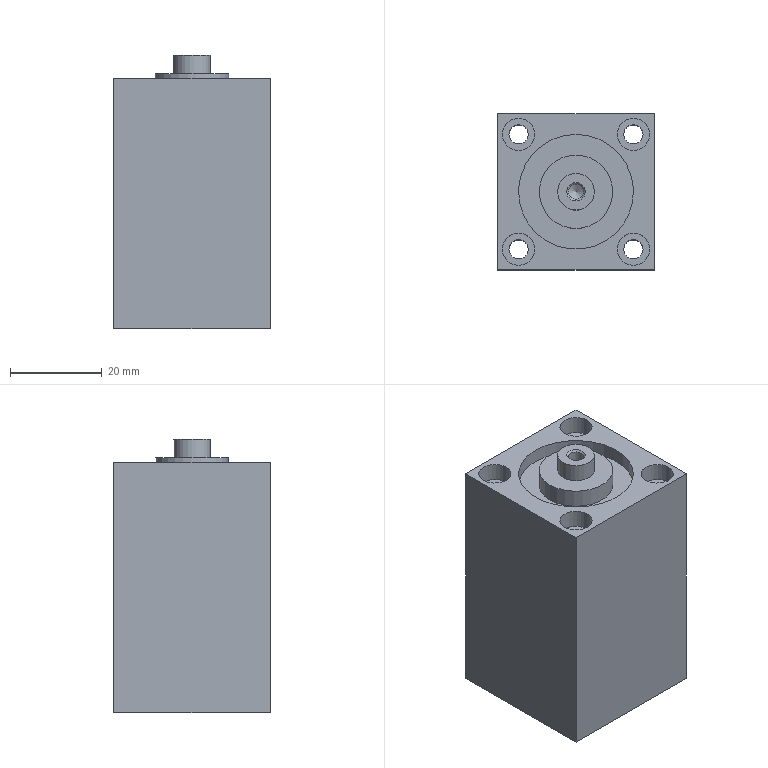Part | NX | features DATUM_CSYS 8, EXTRUDE 7, SKETCH 7, HOLE PACKAGE 1, Instance Feature 1, Mirror Feature 1, SIMPLE HOLE 1, SUBTRACT 1, SYMBOLIC_THREAD 1 | 2 solids | 38 faces | box 34 x 34 x 59.5 mm | volume 58620 mm3 | plane 19 | cylinder 17 | cone 2 | commonest cylinder face diameters 7 x8 4.2 x4 8 x2 3.3 x1 16 x1 25 x1
STEP:
#1=CARTESIAN_POINT('',(4.,0.,59.5));
#2=VERTEX_POINT('',#1);
#3=CARTESIAN_POINT('',(0.,0.,59.5));
#4=DIRECTION('',(0.,0.,1.));
#5=DIRECTION('',(1.,0.,0.));
#6=AXIS2_PLACEMENT_3D('',#3,#4,#5);
#7=CIRCLE('',#6,4.);
#8=EDGE_CURVE('',#2,#2,#7,.T.);
#9=ORIENTED_EDGE('',*,*,#8,.F.);
#10=EDGE_LOOP('',(#9));
#11=FACE_BOUND('',#10,.T.);
#12=CARTESIAN_POINT('',(4.,0.,5.5));
#13=VERTEX_POINT('',#12);
#14=CARTESIAN_POINT('',(0.,0.,5.5));
#15=DIRECTION('',(0.,0.,1.));
#16=DIRECTION('',(1.,0.,0.));
#17=AXIS2_PLACEMENT_3D('',#14,#15,#16);
#18=CIRCLE('',#17,4.);
#19=EDGE_CURVE('',#13,#13,#18,.T.);
#20=ORIENTED_EDGE('',*,*,#19,.T.);
#21=EDGE_LOOP('',(#20));
#22=FACE_BOUND('',#21,.T.);
#23=CARTESIAN_POINT('',(0.,0.,59.5));
#24=DIRECTION('',(0.,0.,-1.));
#25=DIRECTION('',(-1.,0.,0.));
#26=AXIS2_PLACEMENT_3D('',#23,#24,#25);
#27=CYLINDRICAL_SURFACE('',#26,4.);
#28=ADVANCED_FACE('',(#11,#22),#27,.T.);
#29=CARTESIAN_POINT('',(2.,0.,59.5));
#30=VERTEX_POINT('',#29);
#31=CARTESIAN_POINT('',(0.,0.,59.5));
#32=DIRECTION('',(0.,0.,1.));
#33=DIRECTION('',(1.,0.,0.));
#34=AXIS2_PLACEMENT_3D('',#31,#32,#33);
#35=CIRCLE('',#34,2.);
#36=EDGE_CURVE('',#30,#30,#35,.F.);
#37=ORIENTED_EDGE('',*,*,#36,.T.);
#38=EDGE_LOOP('',(#37));
#39=FACE_BOUND('',#38,.T.);
#40=ORIENTED_EDGE('',*,*,#8,.T.);
#41=EDGE_LOOP('',(#40));
#42=FACE_BOUND('',#41,.T.);
#43=CARTESIAN_POINT('',(0.,0.,59.5));
#44=DIRECTION('',(0.,0.,1.));
#45=DIRECTION('',(1.,0.,0.));
#46=AXIS2_PLACEMENT_3D('',#43,#44,#45);
#47=PLANE('',#46);
#48=ADVANCED_FACE('',(#39,#42),#47,.T.);
#49=ORIENTED_EDGE('',*,*,#19,.F.);
#50=EDGE_LOOP('',(#49));
#51=FACE_BOUND('',#50,.T.);
#52=CARTESIAN_POINT('',(0.,0.,5.5));
#53=DIRECTION('',(0.,0.,1.));
#54=DIRECTION('',(1.,0.,0.));
#55=AXIS2_PLACEMENT_3D('',#52,#53,#54);
#56=PLANE('',#55);
#57=ADVANCED_FACE('',(#51),#56,.F.);
#58=CARTESIAN_POINT('',(-1.65,0.,47.5));
#59=VERTEX_POINT('',#58);
#60=CARTESIAN_POINT('',(0.,0.,47.5));
#61=DIRECTION('',(0.,0.,-1.));
#62=DIRECTION('',(-1.,0.,0.));
#63=AXIS2_PLACEMENT_3D('',#60,#61,#62);
#64=CIRCLE('',#63,1.65);
#65=EDGE_CURVE('',#59,#59,#64,.F.);
#66=ORIENTED_EDGE('',*,*,#65,.T.);
#67=EDGE_LOOP('',(#66));
#68=FACE_BOUND('',#67,.T.);
#69=CARTESIAN_POINT('',(0.,0.,46.509));
#70=VERTEX_POINT('',#69);
#71=VERTEX_LOOP('',#70);
#72=FACE_BOUND('',#71,.T.);
#73=CARTESIAN_POINT('',(0.,0.,47.5));
#74=DIRECTION('',(0.,0.,1.));
#75=DIRECTION('',(1.,0.,0.));
#76=AXIS2_PLACEMENT_3D('',#73,#74,#75);
#77=CONICAL_SURFACE('',#76,1.65,1.03);
#78=ADVANCED_FACE('',(#68,#72),#77,.F.);
#79=CARTESIAN_POINT('',(1.65,0.,59.15));
#80=VERTEX_POINT('',#79);
#81=CARTESIAN_POINT('',(0.,0.,59.15));
#82=DIRECTION('',(0.,0.,1.));
#83=DIRECTION('',(1.,0.,0.));
#84=AXIS2_PLACEMENT_3D('',#81,#82,#83);
#85=CIRCLE('',#84,1.65);
#86=EDGE_CURVE('',#80,#80,#85,.T.);
#87=ORIENTED_EDGE('',*,*,#86,.T.);
#88=EDGE_LOOP('',(#87));
#89=FACE_BOUND('',#88,.T.);
#90=ORIENTED_EDGE('',*,*,#65,.F.);
#91=EDGE_LOOP('',(#90));
#92=FACE_BOUND('',#91,.T.);
#93=CARTESIAN_POINT('',(0.,0.,59.5));
#94=DIRECTION('',(0.,0.,-1.));
#95=DIRECTION('',(-1.,0.,0.));
#96=AXIS2_PLACEMENT_3D('',#93,#94,#95);
#97=CYLINDRICAL_SURFACE('',#96,1.65);
#98=ADVANCED_FACE('',(#89,#92),#97,.F.);
#99=ORIENTED_EDGE('',*,*,#86,.F.);
#100=EDGE_LOOP('',(#99));
#101=FACE_BOUND('',#100,.T.);
#102=ORIENTED_EDGE('',*,*,#36,.F.);
#103=EDGE_LOOP('',(#102));
#104=FACE_BOUND('',#103,.T.);
#105=CARTESIAN_POINT('',(0.,0.,59.5));
#106=DIRECTION('',(0.,0.,1.));
#107=DIRECTION('',(1.,0.,0.));
#108=AXIS2_PLACEMENT_3D('',#105,#106,#107);
#109=CONICAL_SURFACE('',#108,2.,0.7854);
#110=ADVANCED_FACE('',(#101,#104),#109,.F.);
#111=CLOSED_SHELL('',(#28,#48,#57,#78,#98,#110));
#112=MANIFOLD_SOLID_BREP('',#111);
#113=CARTESIAN_POINT('',(-16.,12.5,54.5));
#114=VERTEX_POINT('',#113);
#115=CARTESIAN_POINT('',(-12.5,12.5,54.5));
#116=DIRECTION('',(0.,0.,-1.));
#117=DIRECTION('',(-1.,0.,0.));
#118=AXIS2_PLACEMENT_3D('',#115,#116,#117);
#119=CIRCLE('',#118,3.5);
#120=EDGE_CURVE('',#114,#114,#119,.T.);
#121=ORIENTED_EDGE('',*,*,#120,.T.);
#122=EDGE_LOOP('',(#121));
#123=FACE_BOUND('',#122,.T.);
#124=CARTESIAN_POINT('',(16.,12.5,54.5));
#125=VERTEX_POINT('',#124);
#126=CARTESIAN_POINT('',(12.5,12.5,54.5));
#127=DIRECTION('',(0.,0.,1.));
#128=DIRECTION('',(1.,0.,0.));
#129=AXIS2_PLACEMENT_3D('',#126,#127,#128);
#130=CIRCLE('',#129,3.5);
#131=EDGE_CURVE('',#125,#125,#130,.T.);
#132=ORIENTED_EDGE('',*,*,#131,.F.);
#133=EDGE_LOOP('',(#132));
#134=FACE_BOUND('',#133,.T.);
#135=CARTESIAN_POINT('',(0.,12.5,54.5));
#136=VERTEX_POINT('',#135);
#137=CARTESIAN_POINT('',(0.,0.,54.5));
#138=DIRECTION('',(0.,0.,1.));
#139=DIRECTION('',(0.,1.,0.));
#140=AXIS2_PLACEMENT_3D('',#137,#138,#139);
#141=CIRCLE('',#140,12.5);
#142=EDGE_CURVE('',#136,#136,#141,.T.);
#143=ORIENTED_EDGE('',*,*,#142,.F.);
#144=EDGE_LOOP('',(#143));
#145=FACE_BOUND('',#144,.T.);
#146=CARTESIAN_POINT('',(-17.,17.,54.5));
#147=VERTEX_POINT('',#146);
#148=CARTESIAN_POINT('',(-17.,-17.,54.5));
#149=VERTEX_POINT('',#148);
#150=CARTESIAN_POINT('',(-17.,17.,54.5));
#151=DIRECTION('',(0.,-1.,0.));
#152=VECTOR('',#151,1000.);
#153=LINE('',#150,#152);
#154=EDGE_CURVE('',#147,#149,#153,.T.);
#155=ORIENTED_EDGE('',*,*,#154,.T.);
#156=CARTESIAN_POINT('',(17.,-17.,54.5));
#157=VERTEX_POINT('',#156);
#158=CARTESIAN_POINT('',(-17.,-17.,54.5));
#159=DIRECTION('',(1.,0.,0.));
#160=VECTOR('',#159,1000.);
#161=LINE('',#158,#160);
#162=EDGE_CURVE('',#149,#157,#161,.T.);
#163=ORIENTED_EDGE('',*,*,#162,.T.);
#164=CARTESIAN_POINT('',(17.,17.,54.5));
#165=VERTEX_POINT('',#164);
#166=CARTESIAN_POINT('',(17.,-17.,54.5));
#167=DIRECTION('',(0.,1.,0.));
#168=VECTOR('',#167,1000.);
#169=LINE('',#166,#168);
#170=EDGE_CURVE('',#157,#165,#169,.T.);
#171=ORIENTED_EDGE('',*,*,#170,.T.);
#172=CARTESIAN_POINT('',(17.,17.,54.5));
#173=DIRECTION('',(-1.,0.,0.));
#174=VECTOR('',#173,1000.);
#175=LINE('',#172,#174);
#176=EDGE_CURVE('',#165,#147,#175,.T.);
#177=ORIENTED_EDGE('',*,*,#176,.T.);
#178=EDGE_LOOP('',(#155,#163,#171,#177));
#179=FACE_BOUND('',#178,.T.);
#180=CARTESIAN_POINT('',(-16.,-12.5,54.5));
#181=VERTEX_POINT('',#180);
#182=CARTESIAN_POINT('',(-12.5,-12.5,54.5));
#183=DIRECTION('',(0.,0.,1.));
#184=DIRECTION('',(-1.,0.,0.));
#185=AXIS2_PLACEMENT_3D('',#182,#183,#184);
#186=CIRCLE('',#185,3.5);
#187=EDGE_CURVE('',#181,#181,#186,.T.);
#188=ORIENTED_EDGE('',*,*,#187,.F.);
#189=EDGE_LOOP('',(#188));
#190=FACE_BOUND('',#189,.T.);
#191=CARTESIAN_POINT('',(16.,-12.5,54.5));
#192=VERTEX_POINT('',#191);
#193=CARTESIAN_POINT('',(12.5,-12.5,54.5));
#194=DIRECTION('',(0.,0.,-1.));
#195=DIRECTION('',(1.,0.,0.));
#196=AXIS2_PLACEMENT_3D('',#193,#194,#195);
#197=CIRCLE('',#196,3.5);
#198=EDGE_CURVE('',#192,#192,#197,.T.);
#199=ORIENTED_EDGE('',*,*,#198,.T.);
#200=EDGE_LOOP('',(#199));
#201=FACE_BOUND('',#200,.T.);
#202=CARTESIAN_POINT('',(0.,0.,54.5));
#203=DIRECTION('',(0.,0.,1.));
#204=DIRECTION('',(1.,0.,0.));
#205=AXIS2_PLACEMENT_3D('',#202,#203,#204);
#206=PLANE('',#205);
#207=ADVANCED_FACE('',(#123,#134,#145,#179,#190,#201),#206,.T.);
#208=CARTESIAN_POINT('',(-16.,12.5,0.));
#209=VERTEX_POINT('',#208);
#210=CARTESIAN_POINT('',(-12.5,12.5,0.));
#211=DIRECTION('',(0.,0.,-1.));
#212=DIRECTION('',(-1.,0.,0.));
#213=AXIS2_PLACEMENT_3D('',#210,#211,#212);
#214=CIRCLE('',#213,3.5);
#215=EDGE_CURVE('',#209,#209,#214,.T.);
#216=ORIENTED_EDGE('',*,*,#215,.F.);
#217=EDGE_LOOP('',(#216));
#218=FACE_BOUND('',#217,.T.);
#219=CARTESIAN_POINT('',(16.,12.5,0.));
#220=VERTEX_POINT('',#219);
#221=CARTESIAN_POINT('',(12.5,12.5,0.));
#222=DIRECTION('',(0.,0.,1.));
#223=DIRECTION('',(1.,0.,0.));
#224=AXIS2_PLACEMENT_3D('',#221,#222,#223);
#225=CIRCLE('',#224,3.5);
#226=EDGE_CURVE('',#220,#220,#225,.T.);
#227=ORIENTED_EDGE('',*,*,#226,.T.);
#228=EDGE_LOOP('',(#227));
#229=FACE_BOUND('',#228,.T.);
#230=CARTESIAN_POINT('',(-17.,17.,0.));
#231=VERTEX_POINT('',#230);
#232=CARTESIAN_POINT('',(-17.,-17.,0.));
#233=VERTEX_POINT('',#232);
#234=CARTESIAN_POINT('',(-17.,17.,0.));
#235=DIRECTION('',(0.,-1.,0.));
#236=VECTOR('',#235,1000.);
#237=LINE('',#234,#236);
#238=EDGE_CURVE('',#231,#233,#237,.T.);
#239=ORIENTED_EDGE('',*,*,#238,.F.);
#240=CARTESIAN_POINT('',(17.,17.,0.));
#241=VERTEX_POINT('',#240);
#242=CARTESIAN_POINT('',(17.,17.,0.));
#243=DIRECTION('',(-1.,0.,0.));
#244=VECTOR('',#243,1000.);
#245=LINE('',#242,#244);
#246=EDGE_CURVE('',#241,#231,#245,.T.);
#247=ORIENTED_EDGE('',*,*,#246,.F.);
#248=CARTESIAN_POINT('',(17.,-17.,0.));
#249=VERTEX_POINT('',#248);
#250=CARTESIAN_POINT('',(17.,-17.,0.));
#251=DIRECTION('',(0.,1.,0.));
#252=VECTOR('',#251,1000.);
#253=LINE('',#250,#252);
#254=EDGE_CURVE('',#249,#241,#253,.T.);
#255=ORIENTED_EDGE('',*,*,#254,.F.);
#256=CARTESIAN_POINT('',(-17.,-17.,0.));
#257=DIRECTION('',(1.,0.,0.));
#258=VECTOR('',#257,1000.);
#259=LINE('',#256,#258);
#260=EDGE_CURVE('',#233,#249,#259,.T.);
#261=ORIENTED_EDGE('',*,*,#260,.F.);
#262=EDGE_LOOP('',(#239,#247,#255,#261));
#263=FACE_BOUND('',#262,.T.);
#264=CARTESIAN_POINT('',(-16.,-12.5,0.));
#265=VERTEX_POINT('',#264);
#266=CARTESIAN_POINT('',(-12.5,-12.5,0.));
#267=DIRECTION('',(0.,0.,1.));
#268=DIRECTION('',(-1.,0.,0.));
#269=AXIS2_PLACEMENT_3D('',#266,#267,#268);
#270=CIRCLE('',#269,3.5);
#271=EDGE_CURVE('',#265,#265,#270,.T.);
#272=ORIENTED_EDGE('',*,*,#271,.T.);
#273=EDGE_LOOP('',(#272));
#274=FACE_BOUND('',#273,.T.);
#275=CARTESIAN_POINT('',(16.,-12.5,0.));
#276=VERTEX_POINT('',#275);
#277=CARTESIAN_POINT('',(12.5,-12.5,0.));
#278=DIRECTION('',(0.,0.,-1.));
#279=DIRECTION('',(1.,0.,0.));
#280=AXIS2_PLACEMENT_3D('',#277,#278,#279);
#281=CIRCLE('',#280,3.5);
#282=EDGE_CURVE('',#276,#276,#281,.T.);
#283=ORIENTED_EDGE('',*,*,#282,.F.);
#284=EDGE_LOOP('',(#283));
#285=FACE_BOUND('',#284,.T.);
#286=CARTESIAN_POINT('',(0.,0.,0.));
#287=DIRECTION('',(0.,0.,1.));
#288=DIRECTION('',(1.,0.,0.));
#289=AXIS2_PLACEMENT_3D('',#286,#287,#288);
#290=PLANE('',#289);
#291=ADVANCED_FACE('',(#218,#229,#263,#274,#285),#290,.F.);
#292=ORIENTED_EDGE('',*,*,#238,.T.);
#293=CARTESIAN_POINT('',(-17.,-17.,54.5));
#294=DIRECTION('',(0.,0.,-1.));
#295=VECTOR('',#294,1000.);
#296=LINE('',#293,#295);
#297=EDGE_CURVE('',#149,#233,#296,.T.);
#298=ORIENTED_EDGE('',*,*,#297,.F.);
#299=ORIENTED_EDGE('',*,*,#154,.F.);
#300=CARTESIAN_POINT('',(-17.,17.,54.5));
#301=DIRECTION('',(0.,0.,-1.));
#302=VECTOR('',#301,1000.);
#303=LINE('',#300,#302);
#304=EDGE_CURVE('',#147,#231,#303,.T.);
#305=ORIENTED_EDGE('',*,*,#304,.T.);
#306=EDGE_LOOP('',(#292,#298,#299,#305));
#307=FACE_BOUND('',#306,.T.);
#308=CARTESIAN_POINT('',(-17.,17.,54.5));
#309=DIRECTION('',(1.,0.,0.));
#310=DIRECTION('',(0.,0.,-1.));
#311=AXIS2_PLACEMENT_3D('',#308,#309,#310);
#312=PLANE('',#311);
#313=ADVANCED_FACE('',(#307),#312,.F.);
#314=ORIENTED_EDGE('',*,*,#260,.T.);
#315=CARTESIAN_POINT('',(17.,-17.,54.5));
#316=DIRECTION('',(0.,0.,-1.));
#317=VECTOR('',#316,1000.);
#318=LINE('',#315,#317);
#319=EDGE_CURVE('',#157,#249,#318,.T.);
#320=ORIENTED_EDGE('',*,*,#319,.F.);
#321=ORIENTED_EDGE('',*,*,#162,.F.);
#322=ORIENTED_EDGE('',*,*,#297,.T.);
#323=EDGE_LOOP('',(#314,#320,#321,#322));
#324=FACE_BOUND('',#323,.T.);
#325=CARTESIAN_POINT('',(-17.,-17.,54.5));
#326=DIRECTION('',(0.,1.,0.));
#327=DIRECTION('',(0.,0.,1.));
#328=AXIS2_PLACEMENT_3D('',#325,#326,#327);
#329=PLANE('',#328);
#330=ADVANCED_FACE('',(#324),#329,.F.);
#331=ORIENTED_EDGE('',*,*,#254,.T.);
#332=CARTESIAN_POINT('',(17.,17.,54.5));
#333=DIRECTION('',(0.,0.,-1.));
#334=VECTOR('',#333,1000.);
#335=LINE('',#332,#334);
#336=EDGE_CURVE('',#165,#241,#335,.T.);
#337=ORIENTED_EDGE('',*,*,#336,.F.);
#338=ORIENTED_EDGE('',*,*,#170,.F.);
#339=ORIENTED_EDGE('',*,*,#319,.T.);
#340=EDGE_LOOP('',(#331,#337,#338,#339));
#341=FACE_BOUND('',#340,.T.);
#342=CARTESIAN_POINT('',(17.,-17.,54.5));
#343=DIRECTION('',(-1.,0.,0.));
#344=DIRECTION('',(0.,0.,1.));
#345=AXIS2_PLACEMENT_3D('',#342,#343,#344);
#346=PLANE('',#345);
#347=ADVANCED_FACE('',(#341),#346,.F.);
#348=ORIENTED_EDGE('',*,*,#246,.T.);
#349=ORIENTED_EDGE('',*,*,#304,.F.);
#350=ORIENTED_EDGE('',*,*,#176,.F.);
#351=ORIENTED_EDGE('',*,*,#336,.T.);
#352=EDGE_LOOP('',(#348,#349,#350,#351));
#353=FACE_BOUND('',#352,.T.);
#354=CARTESIAN_POINT('',(17.,17.,54.5));
#355=DIRECTION('',(0.,-1.,0.));
#356=DIRECTION('',(0.,0.,-1.));
#357=AXIS2_PLACEMENT_3D('',#354,#355,#356);
#358=PLANE('',#357);
#359=ADVANCED_FACE('',(#353),#358,.F.);
#360=CARTESIAN_POINT('',(0.,12.5,51.5));
#361=VERTEX_POINT('',#360);
#362=CARTESIAN_POINT('',(0.,0.,51.5));
#363=DIRECTION('',(0.,0.,1.));
#364=DIRECTION('',(0.,1.,0.));
#365=AXIS2_PLACEMENT_3D('',#362,#363,#364);
#366=CIRCLE('',#365,12.5);
#367=EDGE_CURVE('',#361,#361,#366,.F.);
#368=ORIENTED_EDGE('',*,*,#367,.T.);
#369=EDGE_LOOP('',(#368));
#370=FACE_BOUND('',#369,.T.);
#371=ORIENTED_EDGE('',*,*,#142,.T.);
#372=EDGE_LOOP('',(#371));
#373=FACE_BOUND('',#372,.T.);
#374=CARTESIAN_POINT('',(0.,0.,51.5));
#375=DIRECTION('',(0.,0.,1.));
#376=DIRECTION('',(1.,0.,0.));
#377=AXIS2_PLACEMENT_3D('',#374,#375,#376);
#378=CYLINDRICAL_SURFACE('',#377,12.5);
#379=ADVANCED_FACE('',(#370,#373),#378,.F.);
#380=CARTESIAN_POINT('',(8.,0.,51.5));
#381=VERTEX_POINT('',#380);
#382=CARTESIAN_POINT('',(0.,0.,51.5));
#383=DIRECTION('',(0.,0.,1.));
#384=DIRECTION('',(1.,0.,0.));
#385=AXIS2_PLACEMENT_3D('',#382,#383,#384);
#386=CIRCLE('',#385,8.);
#387=EDGE_CURVE('',#381,#381,#386,.T.);
#388=ORIENTED_EDGE('',*,*,#387,.F.);
#389=EDGE_LOOP('',(#388));
#390=FACE_BOUND('',#389,.T.);
#391=ORIENTED_EDGE('',*,*,#367,.F.);
#392=EDGE_LOOP('',(#391));
#393=FACE_BOUND('',#392,.T.);
#394=CARTESIAN_POINT('',(0.,0.,51.5));
#395=DIRECTION('',(0.,0.,1.));
#396=DIRECTION('',(1.,0.,0.));
#397=AXIS2_PLACEMENT_3D('',#394,#395,#396);
#398=PLANE('',#397);
#399=ADVANCED_FACE('',(#390,#393),#398,.T.);
#400=CARTESIAN_POINT('',(8.,0.,55.5));
#401=VERTEX_POINT('',#400);
#402=CARTESIAN_POINT('',(0.,0.,55.5));
#403=DIRECTION('',(0.,0.,1.));
#404=DIRECTION('',(1.,0.,0.));
#405=AXIS2_PLACEMENT_3D('',#402,#403,#404);
#406=CIRCLE('',#405,8.);
#407=EDGE_CURVE('',#401,#401,#406,.T.);
#408=ORIENTED_EDGE('',*,*,#407,.F.);
#409=EDGE_LOOP('',(#408));
#410=FACE_BOUND('',#409,.T.);
#411=ORIENTED_EDGE('',*,*,#387,.T.);
#412=EDGE_LOOP('',(#411));
#413=FACE_BOUND('',#412,.T.);
#414=CARTESIAN_POINT('',(0.,0.,55.5));
#415=DIRECTION('',(0.,0.,-1.));
#416=DIRECTION('',(-1.,0.,0.));
#417=AXIS2_PLACEMENT_3D('',#414,#415,#416);
#418=CYLINDRICAL_SURFACE('',#417,8.);
#419=ADVANCED_FACE('',(#410,#413),#418,.T.);
#420=CARTESIAN_POINT('',(4.,0.,55.5));
#421=VERTEX_POINT('',#420);
#422=CARTESIAN_POINT('',(0.,0.,55.5));
#423=DIRECTION('',(0.,0.,1.));
#424=DIRECTION('',(1.,0.,0.));
#425=AXIS2_PLACEMENT_3D('',#422,#423,#424);
#426=CIRCLE('',#425,4.);
#427=EDGE_CURVE('',#421,#421,#426,.F.);
#428=ORIENTED_EDGE('',*,*,#427,.T.);
#429=EDGE_LOOP('',(#428));
#430=FACE_BOUND('',#429,.T.);
#431=ORIENTED_EDGE('',*,*,#407,.T.);
#432=EDGE_LOOP('',(#431));
#433=FACE_BOUND('',#432,.T.);
#434=CARTESIAN_POINT('',(0.,0.,55.5));
#435=DIRECTION('',(0.,0.,1.));
#436=DIRECTION('',(1.,0.,0.));
#437=AXIS2_PLACEMENT_3D('',#434,#435,#436);
#438=PLANE('',#437);
#439=ADVANCED_FACE('',(#430,#433),#438,.T.);
#440=CARTESIAN_POINT('',(16.,12.5,4.));
#441=VERTEX_POINT('',#440);
#442=CARTESIAN_POINT('',(12.5,12.5,4.));
#443=DIRECTION('',(0.,0.,1.));
#444=DIRECTION('',(1.,0.,0.));
#445=AXIS2_PLACEMENT_3D('',#442,#443,#444);
#446=CIRCLE('',#445,3.5);
#447=EDGE_CURVE('',#441,#441,#446,.F.);
#448=ORIENTED_EDGE('',*,*,#447,.F.);
#449=EDGE_LOOP('',(#448));
#450=FACE_BOUND('',#449,.T.);
#451=ORIENTED_EDGE('',*,*,#226,.F.);
#452=EDGE_LOOP('',(#451));
#453=FACE_BOUND('',#452,.T.);
#454=CARTESIAN_POINT('',(12.5,12.5,4.));
#455=DIRECTION('',(0.,0.,-1.));
#456=DIRECTION('',(-1.,0.,0.));
#457=AXIS2_PLACEMENT_3D('',#454,#455,#456);
#458=CYLINDRICAL_SURFACE('',#457,3.5);
#459=ADVANCED_FACE('',(#450,#453),#458,.F.);
#460=CARTESIAN_POINT('',(14.6,12.5,4.));
#461=VERTEX_POINT('',#460);
#462=CARTESIAN_POINT('',(12.5,12.5,4.));
#463=DIRECTION('',(0.,0.,1.));
#464=DIRECTION('',(1.,0.,0.));
#465=AXIS2_PLACEMENT_3D('',#462,#463,#464);
#466=CIRCLE('',#465,2.1);
#467=EDGE_CURVE('',#461,#461,#466,.T.);
#468=ORIENTED_EDGE('',*,*,#467,.T.);
#469=EDGE_LOOP('',(#468));
#470=FACE_BOUND('',#469,.T.);
#471=ORIENTED_EDGE('',*,*,#447,.T.);
#472=EDGE_LOOP('',(#471));
#473=FACE_BOUND('',#472,.T.);
#474=CARTESIAN_POINT('',(12.5,12.5,4.));
#475=DIRECTION('',(0.,0.,1.));
#476=DIRECTION('',(1.,0.,0.));
#477=AXIS2_PLACEMENT_3D('',#474,#475,#476);
#478=PLANE('',#477);
#479=ADVANCED_FACE('',(#470,#473),#478,.F.);
#480=CARTESIAN_POINT('',(-16.,12.5,4.));
#481=VERTEX_POINT('',#480);
#482=CARTESIAN_POINT('',(-12.5,12.5,4.));
#483=DIRECTION('',(0.,0.,-1.));
#484=DIRECTION('',(-1.,0.,0.));
#485=AXIS2_PLACEMENT_3D('',#482,#483,#484);
#486=CIRCLE('',#485,3.5);
#487=EDGE_CURVE('',#481,#481,#486,.F.);
#488=ORIENTED_EDGE('',*,*,#487,.T.);
#489=EDGE_LOOP('',(#488));
#490=FACE_BOUND('',#489,.T.);
#491=ORIENTED_EDGE('',*,*,#215,.T.);
#492=EDGE_LOOP('',(#491));
#493=FACE_BOUND('',#492,.T.);
#494=CARTESIAN_POINT('',(-12.5,12.5,4.));
#495=DIRECTION('',(0.,0.,-1.));
#496=DIRECTION('',(-1.,0.,0.));
#497=AXIS2_PLACEMENT_3D('',#494,#495,#496);
#498=CYLINDRICAL_SURFACE('',#497,3.5);
#499=ADVANCED_FACE('',(#490,#493),#498,.F.);
#500=CARTESIAN_POINT('',(-14.6,12.5,4.));
#501=VERTEX_POINT('',#500);
#502=CARTESIAN_POINT('',(-12.5,12.5,4.));
#503=DIRECTION('',(0.,0.,-1.));
#504=DIRECTION('',(-1.,0.,0.));
#505=AXIS2_PLACEMENT_3D('',#502,#503,#504);
#506=CIRCLE('',#505,2.1);
#507=EDGE_CURVE('',#501,#501,#506,.T.);
#508=ORIENTED_EDGE('',*,*,#507,.F.);
#509=EDGE_LOOP('',(#508));
#510=FACE_BOUND('',#509,.T.);
#511=ORIENTED_EDGE('',*,*,#487,.F.);
#512=EDGE_LOOP('',(#511));
#513=FACE_BOUND('',#512,.T.);
#514=CARTESIAN_POINT('',(-12.5,12.5,4.));
#515=DIRECTION('',(0.,0.,-1.));
#516=DIRECTION('',(-1.,0.,0.));
#517=AXIS2_PLACEMENT_3D('',#514,#515,#516);
#518=PLANE('',#517);
#519=ADVANCED_FACE('',(#510,#513),#518,.T.);
#520=CARTESIAN_POINT('',(-16.,-12.5,4.));
#521=VERTEX_POINT('',#520);
#522=CARTESIAN_POINT('',(-12.5,-12.5,4.));
#523=DIRECTION('',(0.,0.,1.));
#524=DIRECTION('',(-1.,0.,0.));
#525=AXIS2_PLACEMENT_3D('',#522,#523,#524);
#526=CIRCLE('',#525,3.5);
#527=EDGE_CURVE('',#521,#521,#526,.F.);
#528=ORIENTED_EDGE('',*,*,#527,.F.);
#529=EDGE_LOOP('',(#528));
#530=FACE_BOUND('',#529,.T.);
#531=ORIENTED_EDGE('',*,*,#271,.F.);
#532=EDGE_LOOP('',(#531));
#533=FACE_BOUND('',#532,.T.);
#534=CARTESIAN_POINT('',(-12.5,-12.5,4.));
#535=DIRECTION('',(0.,0.,-1.));
#536=DIRECTION('',(-1.,0.,0.));
#537=AXIS2_PLACEMENT_3D('',#534,#535,#536);
#538=CYLINDRICAL_SURFACE('',#537,3.5);
#539=ADVANCED_FACE('',(#530,#533),#538,.F.);
#540=CARTESIAN_POINT('',(-10.4,-12.5,4.));
#541=VERTEX_POINT('',#540);
#542=CARTESIAN_POINT('',(-12.5,-12.5,4.));
#543=DIRECTION('',(0.,0.,1.));
#544=DIRECTION('',(1.,0.,0.));
#545=AXIS2_PLACEMENT_3D('',#542,#543,#544);
#546=CIRCLE('',#545,2.1);
#547=EDGE_CURVE('',#541,#541,#546,.T.);
#548=ORIENTED_EDGE('',*,*,#547,.T.);
#549=EDGE_LOOP('',(#548));
#550=FACE_BOUND('',#549,.T.);
#551=ORIENTED_EDGE('',*,*,#527,.T.);
#552=EDGE_LOOP('',(#551));
#553=FACE_BOUND('',#552,.T.);
#554=CARTESIAN_POINT('',(-12.5,-12.5,4.));
#555=DIRECTION('',(0.,0.,1.));
#556=DIRECTION('',(1.,0.,0.));
#557=AXIS2_PLACEMENT_3D('',#554,#555,#556);
#558=PLANE('',#557);
#559=ADVANCED_FACE('',(#550,#553),#558,.F.);
#560=CARTESIAN_POINT('',(16.,-12.5,4.));
#561=VERTEX_POINT('',#560);
#562=CARTESIAN_POINT('',(12.5,-12.5,4.));
#563=DIRECTION('',(0.,0.,-1.));
#564=DIRECTION('',(1.,0.,0.));
#565=AXIS2_PLACEMENT_3D('',#562,#563,#564);
#566=CIRCLE('',#565,3.5);
#567=EDGE_CURVE('',#561,#561,#566,.F.);
#568=ORIENTED_EDGE('',*,*,#567,.T.);
#569=EDGE_LOOP('',(#568));
#570=FACE_BOUND('',#569,.T.);
#571=ORIENTED_EDGE('',*,*,#282,.T.);
#572=EDGE_LOOP('',(#571));
#573=FACE_BOUND('',#572,.T.);
#574=CARTESIAN_POINT('',(12.5,-12.5,4.));
#575=DIRECTION('',(0.,0.,-1.));
#576=DIRECTION('',(-1.,0.,0.));
#577=AXIS2_PLACEMENT_3D('',#574,#575,#576);
#578=CYLINDRICAL_SURFACE('',#577,3.5);
#579=ADVANCED_FACE('',(#570,#573),#578,.F.);
#580=CARTESIAN_POINT('',(10.4,-12.5,4.));
#581=VERTEX_POINT('',#580);
#582=CARTESIAN_POINT('',(12.5,-12.5,4.));
#583=DIRECTION('',(0.,0.,-1.));
#584=DIRECTION('',(-1.,0.,0.));
#585=AXIS2_PLACEMENT_3D('',#582,#583,#584);
#586=CIRCLE('',#585,2.1);
#587=EDGE_CURVE('',#581,#581,#586,.T.);
#588=ORIENTED_EDGE('',*,*,#587,.F.);
#589=EDGE_LOOP('',(#588));
#590=FACE_BOUND('',#589,.T.);
#591=ORIENTED_EDGE('',*,*,#567,.F.);
#592=EDGE_LOOP('',(#591));
#593=FACE_BOUND('',#592,.T.);
#594=CARTESIAN_POINT('',(12.5,-12.5,4.));
#595=DIRECTION('',(0.,0.,-1.));
#596=DIRECTION('',(-1.,0.,0.));
#597=AXIS2_PLACEMENT_3D('',#594,#595,#596);
#598=PLANE('',#597);
#599=ADVANCED_FACE('',(#590,#593),#598,.T.);
#600=CARTESIAN_POINT('',(16.,12.5,50.5));
#601=VERTEX_POINT('',#600);
#602=CARTESIAN_POINT('',(12.5,12.5,50.5));
#603=DIRECTION('',(0.,0.,1.));
#604=DIRECTION('',(1.,0.,0.));
#605=AXIS2_PLACEMENT_3D('',#602,#603,#604);
#606=CIRCLE('',#605,3.5);
#607=EDGE_CURVE('',#601,#601,#606,.F.);
#608=ORIENTED_EDGE('',*,*,#607,.T.);
#609=EDGE_LOOP('',(#608));
#610=FACE_BOUND('',#609,.T.);
#611=ORIENTED_EDGE('',*,*,#131,.T.);
#612=EDGE_LOOP('',(#611));
#613=FACE_BOUND('',#612,.T.);
#614=CARTESIAN_POINT('',(12.5,12.5,50.5));
#615=DIRECTION('',(0.,0.,1.));
#616=DIRECTION('',(1.,0.,0.));
#617=AXIS2_PLACEMENT_3D('',#614,#615,#616);
#618=CYLINDRICAL_SURFACE('',#617,3.5);
#619=ADVANCED_FACE('',(#610,#613),#618,.F.);
#620=CARTESIAN_POINT('',(14.6,12.5,50.5));
#621=VERTEX_POINT('',#620);
#622=CARTESIAN_POINT('',(12.5,12.5,50.5));
#623=DIRECTION('',(0.,0.,1.));
#624=DIRECTION('',(1.,0.,0.));
#625=AXIS2_PLACEMENT_3D('',#622,#623,#624);
#626=CIRCLE('',#625,2.1);
#627=EDGE_CURVE('',#621,#621,#626,.T.);
#628=ORIENTED_EDGE('',*,*,#627,.F.);
#629=EDGE_LOOP('',(#628));
#630=FACE_BOUND('',#629,.T.);
#631=ORIENTED_EDGE('',*,*,#607,.F.);
#632=EDGE_LOOP('',(#631));
#633=FACE_BOUND('',#632,.T.);
#634=CARTESIAN_POINT('',(12.5,12.5,50.5));
#635=DIRECTION('',(0.,0.,1.));
#636=DIRECTION('',(1.,0.,0.));
#637=AXIS2_PLACEMENT_3D('',#634,#635,#636);
#638=PLANE('',#637);
#639=ADVANCED_FACE('',(#630,#633),#638,.T.);
#640=CARTESIAN_POINT('',(-16.,12.5,50.5));
#641=VERTEX_POINT('',#640);
#642=CARTESIAN_POINT('',(-12.5,12.5,50.5));
#643=DIRECTION('',(0.,0.,-1.));
#644=DIRECTION('',(-1.,0.,0.));
#645=AXIS2_PLACEMENT_3D('',#642,#643,#644);
#646=CIRCLE('',#645,3.5);
#647=EDGE_CURVE('',#641,#641,#646,.F.);
#648=ORIENTED_EDGE('',*,*,#647,.F.);
#649=EDGE_LOOP('',(#648));
#650=FACE_BOUND('',#649,.T.);
#651=ORIENTED_EDGE('',*,*,#120,.F.);
#652=EDGE_LOOP('',(#651));
#653=FACE_BOUND('',#652,.T.);
#654=CARTESIAN_POINT('',(-12.5,12.5,50.5));
#655=DIRECTION('',(0.,0.,1.));
#656=DIRECTION('',(1.,0.,0.));
#657=AXIS2_PLACEMENT_3D('',#654,#655,#656);
#658=CYLINDRICAL_SURFACE('',#657,3.5);
#659=ADVANCED_FACE('',(#650,#653),#658,.F.);
#660=CARTESIAN_POINT('',(-14.6,12.5,50.5));
#661=VERTEX_POINT('',#660);
#662=CARTESIAN_POINT('',(-12.5,12.5,50.5));
#663=DIRECTION('',(0.,0.,-1.));
#664=DIRECTION('',(-1.,0.,0.));
#665=AXIS2_PLACEMENT_3D('',#662,#663,#664);
#666=CIRCLE('',#665,2.1);
#667=EDGE_CURVE('',#661,#661,#666,.T.);
#668=ORIENTED_EDGE('',*,*,#667,.T.);
#669=EDGE_LOOP('',(#668));
#670=FACE_BOUND('',#669,.T.);
#671=ORIENTED_EDGE('',*,*,#647,.T.);
#672=EDGE_LOOP('',(#671));
#673=FACE_BOUND('',#672,.T.);
#674=CARTESIAN_POINT('',(-12.5,12.5,50.5));
#675=DIRECTION('',(0.,0.,-1.));
#676=DIRECTION('',(-1.,0.,0.));
#677=AXIS2_PLACEMENT_3D('',#674,#675,#676);
#678=PLANE('',#677);
#679=ADVANCED_FACE('',(#670,#673),#678,.F.);
#680=CARTESIAN_POINT('',(-16.,-12.5,50.5));
#681=VERTEX_POINT('',#680);
#682=CARTESIAN_POINT('',(-12.5,-12.5,50.5));
#683=DIRECTION('',(0.,0.,1.));
#684=DIRECTION('',(-1.,0.,0.));
#685=AXIS2_PLACEMENT_3D('',#682,#683,#684);
#686=CIRCLE('',#685,3.5);
#687=EDGE_CURVE('',#681,#681,#686,.F.);
#688=ORIENTED_EDGE('',*,*,#687,.T.);
#689=EDGE_LOOP('',(#688));
#690=FACE_BOUND('',#689,.T.);
#691=ORIENTED_EDGE('',*,*,#187,.T.);
#692=EDGE_LOOP('',(#691));
#693=FACE_BOUND('',#692,.T.);
#694=CARTESIAN_POINT('',(-12.5,-12.5,50.5));
#695=DIRECTION('',(0.,0.,1.));
#696=DIRECTION('',(1.,0.,0.));
#697=AXIS2_PLACEMENT_3D('',#694,#695,#696);
#698=CYLINDRICAL_SURFACE('',#697,3.5);
#699=ADVANCED_FACE('',(#690,#693),#698,.F.);
#700=CARTESIAN_POINT('',(-10.4,-12.5,50.5));
#701=VERTEX_POINT('',#700);
#702=CARTESIAN_POINT('',(-12.5,-12.5,50.5));
#703=DIRECTION('',(0.,0.,1.));
#704=DIRECTION('',(1.,0.,0.));
#705=AXIS2_PLACEMENT_3D('',#702,#703,#704);
#706=CIRCLE('',#705,2.1);
#707=EDGE_CURVE('',#701,#701,#706,.T.);
#708=ORIENTED_EDGE('',*,*,#707,.F.);
#709=EDGE_LOOP('',(#708));
#710=FACE_BOUND('',#709,.T.);
#711=ORIENTED_EDGE('',*,*,#687,.F.);
#712=EDGE_LOOP('',(#711));
#713=FACE_BOUND('',#712,.T.);
#714=CARTESIAN_POINT('',(-12.5,-12.5,50.5));
#715=DIRECTION('',(0.,0.,1.));
#716=DIRECTION('',(1.,0.,0.));
#717=AXIS2_PLACEMENT_3D('',#714,#715,#716);
#718=PLANE('',#717);
#719=ADVANCED_FACE('',(#710,#713),#718,.T.);
#720=CARTESIAN_POINT('',(16.,-12.5,50.5));
#721=VERTEX_POINT('',#720);
#722=CARTESIAN_POINT('',(12.5,-12.5,50.5));
#723=DIRECTION('',(0.,0.,-1.));
#724=DIRECTION('',(1.,0.,0.));
#725=AXIS2_PLACEMENT_3D('',#722,#723,#724);
#726=CIRCLE('',#725,3.5);
#727=EDGE_CURVE('',#721,#721,#726,.F.);
#728=ORIENTED_EDGE('',*,*,#727,.F.);
#729=EDGE_LOOP('',(#728));
#730=FACE_BOUND('',#729,.T.);
#731=ORIENTED_EDGE('',*,*,#198,.F.);
#732=EDGE_LOOP('',(#731));
#733=FACE_BOUND('',#732,.T.);
#734=CARTESIAN_POINT('',(12.5,-12.5,50.5));
#735=DIRECTION('',(0.,0.,1.));
#736=DIRECTION('',(1.,0.,0.));
#737=AXIS2_PLACEMENT_3D('',#734,#735,#736);
#738=CYLINDRICAL_SURFACE('',#737,3.5);
#739=ADVANCED_FACE('',(#730,#733),#738,.F.);
#740=CARTESIAN_POINT('',(10.4,-12.5,50.5));
#741=VERTEX_POINT('',#740);
#742=CARTESIAN_POINT('',(12.5,-12.5,50.5));
#743=DIRECTION('',(0.,0.,-1.));
#744=DIRECTION('',(-1.,0.,0.));
#745=AXIS2_PLACEMENT_3D('',#742,#743,#744);
#746=CIRCLE('',#745,2.1);
#747=EDGE_CURVE('',#741,#741,#746,.T.);
#748=ORIENTED_EDGE('',*,*,#747,.T.);
#749=EDGE_LOOP('',(#748));
#750=FACE_BOUND('',#749,.T.);
#751=ORIENTED_EDGE('',*,*,#727,.T.);
#752=EDGE_LOOP('',(#751));
#753=FACE_BOUND('',#752,.T.);
#754=CARTESIAN_POINT('',(12.5,-12.5,50.5));
#755=DIRECTION('',(0.,0.,-1.));
#756=DIRECTION('',(-1.,0.,0.));
#757=AXIS2_PLACEMENT_3D('',#754,#755,#756);
#758=PLANE('',#757);
#759=ADVANCED_FACE('',(#750,#753),#758,.F.);
#760=ORIENTED_EDGE('',*,*,#587,.T.);
#761=EDGE_LOOP('',(#760));
#762=FACE_BOUND('',#761,.T.);
#763=ORIENTED_EDGE('',*,*,#747,.F.);
#764=EDGE_LOOP('',(#763));
#765=FACE_BOUND('',#764,.T.);
#766=CARTESIAN_POINT('',(12.5,-12.5,-42.5));
#767=DIRECTION('',(0.,0.,1.));
#768=DIRECTION('',(1.,0.,0.));
#769=AXIS2_PLACEMENT_3D('',#766,#767,#768);
#770=CYLINDRICAL_SURFACE('',#769,2.1);
#771=ADVANCED_FACE('',(#762,#765),#770,.F.);
#772=ORIENTED_EDGE('',*,*,#707,.T.);
#773=EDGE_LOOP('',(#772));
#774=FACE_BOUND('',#773,.T.);
#775=ORIENTED_EDGE('',*,*,#547,.F.);
#776=EDGE_LOOP('',(#775));
#777=FACE_BOUND('',#776,.T.);
#778=CARTESIAN_POINT('',(-12.5,-12.5,-42.5));
#779=DIRECTION('',(0.,0.,1.));
#780=DIRECTION('',(1.,0.,0.));
#781=AXIS2_PLACEMENT_3D('',#778,#779,#780);
#782=CYLINDRICAL_SURFACE('',#781,2.1);
#783=ADVANCED_FACE('',(#774,#777),#782,.F.);
#784=ORIENTED_EDGE('',*,*,#507,.T.);
#785=EDGE_LOOP('',(#784));
#786=FACE_BOUND('',#785,.T.);
#787=ORIENTED_EDGE('',*,*,#667,.F.);
#788=EDGE_LOOP('',(#787));
#789=FACE_BOUND('',#788,.T.);
#790=CARTESIAN_POINT('',(-12.5,12.5,-42.5));
#791=DIRECTION('',(0.,0.,1.));
#792=DIRECTION('',(1.,0.,0.));
#793=AXIS2_PLACEMENT_3D('',#790,#791,#792);
#794=CYLINDRICAL_SURFACE('',#793,2.1);
#795=ADVANCED_FACE('',(#786,#789),#794,.F.);
#796=ORIENTED_EDGE('',*,*,#627,.T.);
#797=EDGE_LOOP('',(#796));
#798=FACE_BOUND('',#797,.T.);
#799=ORIENTED_EDGE('',*,*,#467,.F.);
#800=EDGE_LOOP('',(#799));
#801=FACE_BOUND('',#800,.T.);
#802=CARTESIAN_POINT('',(12.5,12.5,-42.5));
#803=DIRECTION('',(0.,0.,1.));
#804=DIRECTION('',(1.,0.,0.));
#805=AXIS2_PLACEMENT_3D('',#802,#803,#804);
#806=CYLINDRICAL_SURFACE('',#805,2.1);
#807=ADVANCED_FACE('',(#798,#801),#806,.F.);
#808=ORIENTED_EDGE('',*,*,#427,.F.);
#809=EDGE_LOOP('',(#808));
#810=FACE_BOUND('',#809,.T.);
#811=CARTESIAN_POINT('',(4.,0.,5.5));
#812=VERTEX_POINT('',#811);
#813=CARTESIAN_POINT('',(0.,0.,5.5));
#814=DIRECTION('',(0.,0.,1.));
#815=DIRECTION('',(1.,0.,0.));
#816=AXIS2_PLACEMENT_3D('',#813,#814,#815);
#817=CIRCLE('',#816,4.);
#818=EDGE_CURVE('',#812,#812,#817,.F.);
#819=ORIENTED_EDGE('',*,*,#818,.T.);
#820=EDGE_LOOP('',(#819));
#821=FACE_BOUND('',#820,.T.);
#822=CARTESIAN_POINT('',(0.,0.,59.5));
#823=DIRECTION('',(0.,0.,-1.));
#824=DIRECTION('',(-1.,0.,0.));
#825=AXIS2_PLACEMENT_3D('',#822,#823,#824);
#826=CYLINDRICAL_SURFACE('',#825,4.);
#827=ADVANCED_FACE('',(#810,#821),#826,.F.);
#828=ORIENTED_EDGE('',*,*,#818,.F.);
#829=EDGE_LOOP('',(#828));
#830=FACE_BOUND('',#829,.T.);
#831=CARTESIAN_POINT('',(0.,0.,5.5));
#832=DIRECTION('',(0.,0.,1.));
#833=DIRECTION('',(1.,0.,0.));
#834=AXIS2_PLACEMENT_3D('',#831,#832,#833);
#835=PLANE('',#834);
#836=ADVANCED_FACE('',(#830),#835,.T.);
#837=CLOSED_SHELL('',(#207,#291,#313,#330,#347,#359,#379,#399,#419,#439,#459,#479,#499,#519,#539,#559,#579,#599,#619,#639,#659,#679,#699,#719,#739,#759,#771,#783,#795,#807,#827,#836));
#838=MANIFOLD_SOLID_BREP('',#837);
#839=(LENGTH_UNIT()NAMED_UNIT(*)SI_UNIT(.MILLI.,.METRE.));
#840=UNCERTAINTY_MEASURE_WITH_UNIT(LENGTH_MEASURE(0.00001),#839,'','');
#841=(NAMED_UNIT(*)PLANE_ANGLE_UNIT()SI_UNIT($,.RADIAN.));
#842=(NAMED_UNIT(*)SI_UNIT($,.STERADIAN.)SOLID_ANGLE_UNIT());
#843=(GEOMETRIC_REPRESENTATION_CONTEXT(3)GLOBAL_UNCERTAINTY_ASSIGNED_CONTEXT((#840))GLOBAL_UNIT_ASSIGNED_CONTEXT((#839,#841,#842))REPRESENTATION_CONTEXT('',''));
#844=ADVANCED_BREP_SHAPE_REPRESENTATION('',(#112,#838),#843);